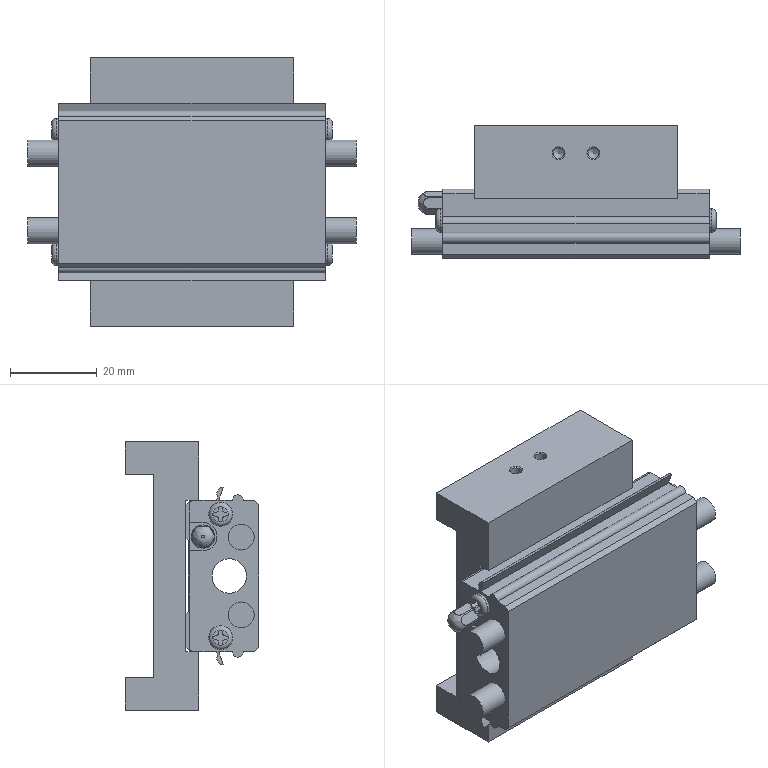Part | STEP file | C-KSC50-B1-1-NS_bl | 1 solid | 298 faces | box 76 x 30.8 x 62 mm | volume 62545 mm3 | plane 205 | cylinder 58 | cone 30 | torus 4 | spline 1 | commonest cylinder face diameters 0.6 x16 2.459 x6 3.242 x5 8 x5 2 x4 5.5 x4